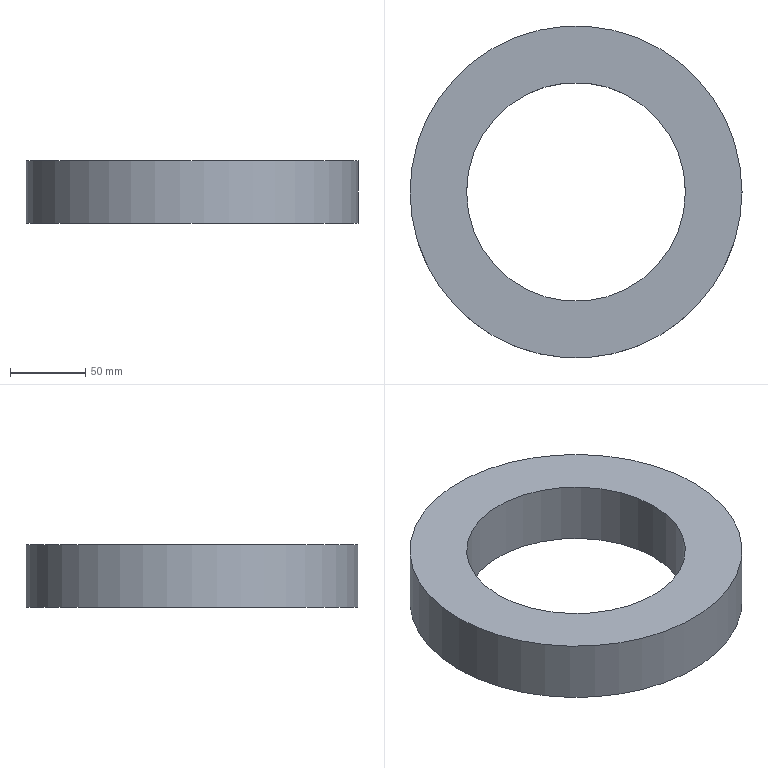Part | NX | features 连杆套筒外 2 | 1 solid | 4 faces | box 220 x 220 x 41.57 mm | volume 893766 mm3 | plane 2 | cylinder 2 | commonest cylinder face diameters 145 x1 220 x1
STEP:
#1=CARTESIAN_POINT('',(110.,0.,41.57));
#2=VERTEX_POINT('',#1);
#3=CARTESIAN_POINT('',(0.,0.,41.57));
#4=DIRECTION('',(0.,0.,1.));
#5=DIRECTION('',(1.,0.,0.));
#6=AXIS2_PLACEMENT_3D('',#3,#4,#5);
#7=CIRCLE('',#6,110.);
#8=EDGE_CURVE('',#2,#2,#7,.T.);
#9=ORIENTED_EDGE('',*,*,#8,.T.);
#10=EDGE_LOOP('',(#9));
#11=FACE_BOUND('',#10,.T.);
#12=CARTESIAN_POINT('',(72.5,0.,41.57));
#13=VERTEX_POINT('',#12);
#14=CARTESIAN_POINT('',(0.,0.,41.57));
#15=DIRECTION('',(0.,0.,1.));
#16=DIRECTION('',(1.,0.,0.));
#17=AXIS2_PLACEMENT_3D('',#14,#15,#16);
#18=CIRCLE('',#17,72.5);
#19=EDGE_CURVE('',#13,#13,#18,.T.);
#20=ORIENTED_EDGE('',*,*,#19,.F.);
#21=EDGE_LOOP('',(#20));
#22=FACE_BOUND('',#21,.T.);
#23=CARTESIAN_POINT('',(0.,0.,41.57));
#24=DIRECTION('',(0.,0.,1.));
#25=DIRECTION('',(1.,0.,0.));
#26=AXIS2_PLACEMENT_3D('',#23,#24,#25);
#27=PLANE('',#26);
#28=ADVANCED_FACE('',(#11,#22),#27,.T.);
#29=CARTESIAN_POINT('',(110.,0.,0.));
#30=VERTEX_POINT('',#29);
#31=CARTESIAN_POINT('',(0.,0.,0.));
#32=DIRECTION('',(0.,0.,1.));
#33=DIRECTION('',(1.,0.,0.));
#34=AXIS2_PLACEMENT_3D('',#31,#32,#33);
#35=CIRCLE('',#34,110.);
#36=EDGE_CURVE('',#30,#30,#35,.T.);
#37=ORIENTED_EDGE('',*,*,#36,.F.);
#38=EDGE_LOOP('',(#37));
#39=FACE_BOUND('',#38,.T.);
#40=CARTESIAN_POINT('',(72.5,0.,0.));
#41=VERTEX_POINT('',#40);
#42=CARTESIAN_POINT('',(0.,0.,0.));
#43=DIRECTION('',(0.,0.,1.));
#44=DIRECTION('',(1.,0.,0.));
#45=AXIS2_PLACEMENT_3D('',#42,#43,#44);
#46=CIRCLE('',#45,72.5);
#47=EDGE_CURVE('',#41,#41,#46,.T.);
#48=ORIENTED_EDGE('',*,*,#47,.T.);
#49=EDGE_LOOP('',(#48));
#50=FACE_BOUND('',#49,.T.);
#51=CARTESIAN_POINT('',(0.,0.,0.));
#52=DIRECTION('',(0.,0.,1.));
#53=DIRECTION('',(1.,0.,0.));
#54=AXIS2_PLACEMENT_3D('',#51,#52,#53);
#55=PLANE('',#54);
#56=ADVANCED_FACE('',(#39,#50),#55,.F.);
#57=ORIENTED_EDGE('',*,*,#8,.F.);
#58=EDGE_LOOP('',(#57));
#59=FACE_BOUND('',#58,.T.);
#60=ORIENTED_EDGE('',*,*,#36,.T.);
#61=EDGE_LOOP('',(#60));
#62=FACE_BOUND('',#61,.T.);
#63=CARTESIAN_POINT('',(0.,0.,41.57));
#64=DIRECTION('',(0.,0.,-1.));
#65=DIRECTION('',(-1.,0.,0.));
#66=AXIS2_PLACEMENT_3D('',#63,#64,#65);
#67=CYLINDRICAL_SURFACE('',#66,110.);
#68=ADVANCED_FACE('',(#59,#62),#67,.T.);
#69=ORIENTED_EDGE('',*,*,#19,.T.);
#70=EDGE_LOOP('',(#69));
#71=FACE_BOUND('',#70,.T.);
#72=ORIENTED_EDGE('',*,*,#47,.F.);
#73=EDGE_LOOP('',(#72));
#74=FACE_BOUND('',#73,.T.);
#75=CARTESIAN_POINT('',(0.,0.,41.57));
#76=DIRECTION('',(0.,0.,-1.));
#77=DIRECTION('',(-1.,0.,0.));
#78=AXIS2_PLACEMENT_3D('',#75,#76,#77);
#79=CYLINDRICAL_SURFACE('',#78,72.5);
#80=ADVANCED_FACE('',(#71,#74),#79,.F.);
#81=CLOSED_SHELL('',(#28,#56,#68,#80));
#82=MANIFOLD_SOLID_BREP('',#81);
#83=(LENGTH_UNIT()NAMED_UNIT(*)SI_UNIT(.MILLI.,.METRE.));
#84=UNCERTAINTY_MEASURE_WITH_UNIT(LENGTH_MEASURE(0.00001),#83,'','');
#85=(NAMED_UNIT(*)PLANE_ANGLE_UNIT()SI_UNIT($,.RADIAN.));
#86=(NAMED_UNIT(*)SI_UNIT($,.STERADIAN.)SOLID_ANGLE_UNIT());
#87=(GEOMETRIC_REPRESENTATION_CONTEXT(3)GLOBAL_UNCERTAINTY_ASSIGNED_CONTEXT((#84))GLOBAL_UNIT_ASSIGNED_CONTEXT((#83,#85,#86))REPRESENTATION_CONTEXT('',''));
#88=ADVANCED_BREP_SHAPE_REPRESENTATION('',(#82),#87);